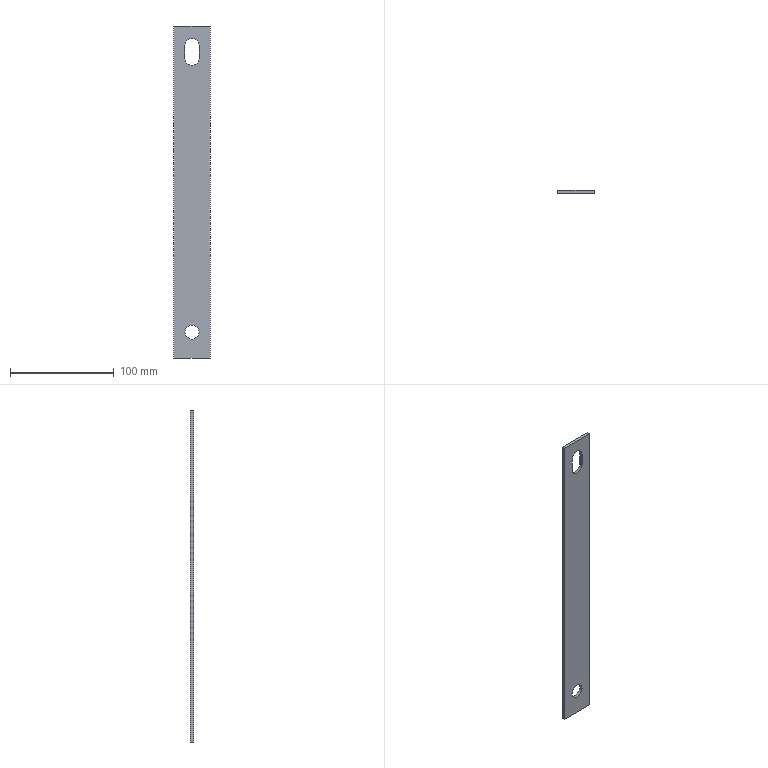Part | NX | features solid 2 | 1 solid | 11 faces | box 35 x 3 x 320 mm | volume 32235 mm3 | plane 8 | cylinder 3 | commonest cylinder face diameters 13.5 x3
STEP:
#1=CARTESIAN_POINT('',(957.5,320.,-165.));
#2=VERTEX_POINT('',#1);
#3=CARTESIAN_POINT('',(922.5,320.,-165.));
#4=VERTEX_POINT('',#3);
#5=CARTESIAN_POINT('',(957.5,320.,-165.));
#6=DIRECTION('',(-1.,0.,0.));
#7=VECTOR('',#6,1000.);
#8=LINE('',#5,#7);
#9=EDGE_CURVE('',#2,#4,#8,.T.);
#10=ORIENTED_EDGE('',*,*,#9,.T.);
#11=CARTESIAN_POINT('',(922.5,323.,-165.));
#12=VERTEX_POINT('',#11);
#13=CARTESIAN_POINT('',(922.5,323.,-165.));
#14=DIRECTION('',(0.,-1.,0.));
#15=VECTOR('',#14,1000.);
#16=LINE('',#13,#15);
#17=EDGE_CURVE('',#12,#4,#16,.T.);
#18=ORIENTED_EDGE('',*,*,#17,.F.);
#19=CARTESIAN_POINT('',(957.5,323.,-165.));
#20=VERTEX_POINT('',#19);
#21=CARTESIAN_POINT('',(957.5,323.,-165.));
#22=DIRECTION('',(-1.,0.,0.));
#23=VECTOR('',#22,1000.);
#24=LINE('',#21,#23);
#25=EDGE_CURVE('',#20,#12,#24,.T.);
#26=ORIENTED_EDGE('',*,*,#25,.F.);
#27=CARTESIAN_POINT('',(957.5,323.,-165.));
#28=DIRECTION('',(0.,-1.,0.));
#29=VECTOR('',#28,1000.);
#30=LINE('',#27,#29);
#31=EDGE_CURVE('',#20,#2,#30,.T.);
#32=ORIENTED_EDGE('',*,*,#31,.T.);
#33=EDGE_LOOP('',(#10,#18,#26,#32));
#34=FACE_BOUND('',#33,.T.);
#35=CARTESIAN_POINT('',(957.5,323.,-165.));
#36=DIRECTION('',(0.,0.,-1.));
#37=DIRECTION('',(0.,1.,0.));
#38=AXIS2_PLACEMENT_3D('',#35,#36,#37);
#39=PLANE('',#38);
#40=ADVANCED_FACE('',(#34),#39,.T.);
#41=CARTESIAN_POINT('',(933.25,323.,-140.));
#42=VERTEX_POINT('',#41);
#43=CARTESIAN_POINT('',(940.,323.,-140.));
#44=DIRECTION('',(0.,1.,0.));
#45=DIRECTION('',(-1.,0.,0.));
#46=AXIS2_PLACEMENT_3D('',#43,#44,#45);
#47=CIRCLE('',#46,6.75);
#48=EDGE_CURVE('',#42,#42,#47,.T.);
#49=ORIENTED_EDGE('',*,*,#48,.T.);
#50=EDGE_LOOP('',(#49));
#51=FACE_BOUND('',#50,.T.);
#52=CARTESIAN_POINT('',(933.25,320.,-140.));
#53=VERTEX_POINT('',#52);
#54=CARTESIAN_POINT('',(940.,320.,-140.));
#55=DIRECTION('',(0.,1.,0.));
#56=DIRECTION('',(-1.,0.,0.));
#57=AXIS2_PLACEMENT_3D('',#54,#55,#56);
#58=CIRCLE('',#57,6.75);
#59=EDGE_CURVE('',#53,#53,#58,.T.);
#60=ORIENTED_EDGE('',*,*,#59,.F.);
#61=EDGE_LOOP('',(#60));
#62=FACE_BOUND('',#61,.T.);
#63=CARTESIAN_POINT('',(940.,323.,-140.));
#64=DIRECTION('',(0.,-1.,0.));
#65=DIRECTION('',(-1.,0.,0.));
#66=AXIS2_PLACEMENT_3D('',#63,#64,#65);
#67=CYLINDRICAL_SURFACE('',#66,6.75);
#68=ADVANCED_FACE('',(#51,#62),#67,.F.);
#69=CARTESIAN_POINT('',(922.5,320.,155.));
#70=VERTEX_POINT('',#69);
#71=CARTESIAN_POINT('',(957.5,320.,155.));
#72=VERTEX_POINT('',#71);
#73=CARTESIAN_POINT('',(922.5,320.,155.));
#74=DIRECTION('',(1.,0.,0.));
#75=VECTOR('',#74,1000.);
#76=LINE('',#73,#75);
#77=EDGE_CURVE('',#70,#72,#76,.T.);
#78=ORIENTED_EDGE('',*,*,#77,.F.);
#79=CARTESIAN_POINT('',(922.5,320.,-85.));
#80=DIRECTION('',(0.,0.,1.));
#81=VECTOR('',#80,1000.);
#82=LINE('',#79,#81);
#83=EDGE_CURVE('',#4,#70,#82,.T.);
#84=ORIENTED_EDGE('',*,*,#83,.F.);
#85=ORIENTED_EDGE('',*,*,#9,.F.);
#86=CARTESIAN_POINT('',(957.5,320.,215.));
#87=DIRECTION('',(0.,0.,-1.));
#88=VECTOR('',#87,1000.);
#89=LINE('',#86,#88);
#90=EDGE_CURVE('',#72,#2,#89,.T.);
#91=ORIENTED_EDGE('',*,*,#90,.F.);
#92=EDGE_LOOP('',(#78,#84,#85,#91));
#93=FACE_BOUND('',#92,.T.);
#94=ORIENTED_EDGE('',*,*,#59,.T.);
#95=EDGE_LOOP('',(#94));
#96=FACE_BOUND('',#95,.T.);
#97=CARTESIAN_POINT('',(933.25,320.,136.25));
#98=VERTEX_POINT('',#97);
#99=CARTESIAN_POINT('',(946.75,320.,136.25));
#100=VERTEX_POINT('',#99);
#101=CARTESIAN_POINT('',(940.,320.,136.25));
#102=DIRECTION('',(0.,1.,0.));
#103=DIRECTION('',(-1.,0.,0.));
#104=AXIS2_PLACEMENT_3D('',#101,#102,#103);
#105=CIRCLE('',#104,6.75);
#106=EDGE_CURVE('',#98,#100,#105,.T.);
#107=ORIENTED_EDGE('',*,*,#106,.T.);
#108=CARTESIAN_POINT('',(946.75,320.,123.75));
#109=VERTEX_POINT('',#108);
#110=CARTESIAN_POINT('',(946.75,320.,123.75));
#111=DIRECTION('',(0.,0.,1.));
#112=VECTOR('',#111,1000.);
#113=LINE('',#110,#112);
#114=EDGE_CURVE('',#109,#100,#113,.T.);
#115=ORIENTED_EDGE('',*,*,#114,.F.);
#116=CARTESIAN_POINT('',(933.25,320.,123.75));
#117=VERTEX_POINT('',#116);
#118=CARTESIAN_POINT('',(940.,320.,123.75));
#119=DIRECTION('',(0.,1.,0.));
#120=DIRECTION('',(-1.,0.,0.));
#121=AXIS2_PLACEMENT_3D('',#118,#119,#120);
#122=CIRCLE('',#121,6.75);
#123=EDGE_CURVE('',#109,#117,#122,.T.);
#124=ORIENTED_EDGE('',*,*,#123,.T.);
#125=CARTESIAN_POINT('',(933.25,320.,136.25));
#126=DIRECTION('',(0.,0.,-1.));
#127=VECTOR('',#126,1000.);
#128=LINE('',#125,#127);
#129=EDGE_CURVE('',#98,#117,#128,.T.);
#130=ORIENTED_EDGE('',*,*,#129,.F.);
#131=EDGE_LOOP('',(#107,#115,#124,#130));
#132=FACE_BOUND('',#131,.T.);
#133=CARTESIAN_POINT('',(922.5,320.,215.));
#134=DIRECTION('',(0.,-1.,0.));
#135=DIRECTION('',(-1.,0.,0.));
#136=AXIS2_PLACEMENT_3D('',#133,#134,#135);
#137=PLANE('',#136);
#138=ADVANCED_FACE('',(#93,#96,#132),#137,.T.);
#139=CARTESIAN_POINT('',(957.5,323.,155.));
#140=VERTEX_POINT('',#139);
#141=CARTESIAN_POINT('',(957.5,323.,215.));
#142=DIRECTION('',(0.,0.,-1.));
#143=VECTOR('',#142,1000.);
#144=LINE('',#141,#143);
#145=EDGE_CURVE('',#140,#20,#144,.T.);
#146=ORIENTED_EDGE('',*,*,#145,.T.);
#147=ORIENTED_EDGE('',*,*,#25,.T.);
#148=CARTESIAN_POINT('',(922.5,323.,155.));
#149=VERTEX_POINT('',#148);
#150=CARTESIAN_POINT('',(922.5,323.,-85.));
#151=DIRECTION('',(0.,0.,1.));
#152=VECTOR('',#151,1000.);
#153=LINE('',#150,#152);
#154=EDGE_CURVE('',#12,#149,#153,.T.);
#155=ORIENTED_EDGE('',*,*,#154,.T.);
#156=CARTESIAN_POINT('',(922.5,323.,155.));
#157=DIRECTION('',(1.,0.,0.));
#158=VECTOR('',#157,1000.);
#159=LINE('',#156,#158);
#160=EDGE_CURVE('',#149,#140,#159,.T.);
#161=ORIENTED_EDGE('',*,*,#160,.T.);
#162=EDGE_LOOP('',(#146,#147,#155,#161));
#163=FACE_BOUND('',#162,.T.);
#164=ORIENTED_EDGE('',*,*,#48,.F.);
#165=EDGE_LOOP('',(#164));
#166=FACE_BOUND('',#165,.T.);
#167=CARTESIAN_POINT('',(933.25,323.,136.25));
#168=VERTEX_POINT('',#167);
#169=CARTESIAN_POINT('',(946.75,323.,136.25));
#170=VERTEX_POINT('',#169);
#171=CARTESIAN_POINT('',(940.,323.,136.25));
#172=DIRECTION('',(0.,1.,0.));
#173=DIRECTION('',(-1.,0.,0.));
#174=AXIS2_PLACEMENT_3D('',#171,#172,#173);
#175=CIRCLE('',#174,6.75);
#176=EDGE_CURVE('',#168,#170,#175,.T.);
#177=ORIENTED_EDGE('',*,*,#176,.F.);
#178=CARTESIAN_POINT('',(933.25,323.,123.75));
#179=VERTEX_POINT('',#178);
#180=CARTESIAN_POINT('',(933.25,323.,136.25));
#181=DIRECTION('',(0.,0.,-1.));
#182=VECTOR('',#181,1000.);
#183=LINE('',#180,#182);
#184=EDGE_CURVE('',#168,#179,#183,.T.);
#185=ORIENTED_EDGE('',*,*,#184,.T.);
#186=CARTESIAN_POINT('',(946.75,323.,123.75));
#187=VERTEX_POINT('',#186);
#188=CARTESIAN_POINT('',(940.,323.,123.75));
#189=DIRECTION('',(0.,1.,0.));
#190=DIRECTION('',(-1.,0.,0.));
#191=AXIS2_PLACEMENT_3D('',#188,#189,#190);
#192=CIRCLE('',#191,6.75);
#193=EDGE_CURVE('',#187,#179,#192,.T.);
#194=ORIENTED_EDGE('',*,*,#193,.F.);
#195=CARTESIAN_POINT('',(946.75,323.,123.75));
#196=DIRECTION('',(0.,0.,1.));
#197=VECTOR('',#196,1000.);
#198=LINE('',#195,#197);
#199=EDGE_CURVE('',#187,#170,#198,.T.);
#200=ORIENTED_EDGE('',*,*,#199,.T.);
#201=EDGE_LOOP('',(#177,#185,#194,#200));
#202=FACE_BOUND('',#201,.T.);
#203=CARTESIAN_POINT('',(922.5,323.,215.));
#204=DIRECTION('',(0.,-1.,0.));
#205=DIRECTION('',(-1.,0.,0.));
#206=AXIS2_PLACEMENT_3D('',#203,#204,#205);
#207=PLANE('',#206);
#208=ADVANCED_FACE('',(#163,#166,#202),#207,.F.);
#209=ORIENTED_EDGE('',*,*,#90,.T.);
#210=ORIENTED_EDGE('',*,*,#31,.F.);
#211=ORIENTED_EDGE('',*,*,#145,.F.);
#212=CARTESIAN_POINT('',(957.5,323.,155.));
#213=DIRECTION('',(0.,-1.,0.));
#214=VECTOR('',#213,1000.);
#215=LINE('',#212,#214);
#216=EDGE_CURVE('',#140,#72,#215,.T.);
#217=ORIENTED_EDGE('',*,*,#216,.T.);
#218=EDGE_LOOP('',(#209,#210,#211,#217));
#219=FACE_BOUND('',#218,.T.);
#220=CARTESIAN_POINT('',(957.5,323.,215.));
#221=DIRECTION('',(1.,0.,0.));
#222=DIRECTION('',(0.,0.,-1.));
#223=AXIS2_PLACEMENT_3D('',#220,#221,#222);
#224=PLANE('',#223);
#225=ADVANCED_FACE('',(#219),#224,.T.);
#226=CARTESIAN_POINT('',(922.5,323.,155.));
#227=DIRECTION('',(0.,-1.,0.));
#228=VECTOR('',#227,1000.);
#229=LINE('',#226,#228);
#230=EDGE_CURVE('',#149,#70,#229,.T.);
#231=ORIENTED_EDGE('',*,*,#230,.F.);
#232=ORIENTED_EDGE('',*,*,#154,.F.);
#233=ORIENTED_EDGE('',*,*,#17,.T.);
#234=ORIENTED_EDGE('',*,*,#83,.T.);
#235=EDGE_LOOP('',(#231,#232,#233,#234));
#236=FACE_BOUND('',#235,.T.);
#237=CARTESIAN_POINT('',(922.5,323.,-85.));
#238=DIRECTION('',(-1.,0.,0.));
#239=DIRECTION('',(0.,0.,1.));
#240=AXIS2_PLACEMENT_3D('',#237,#238,#239);
#241=PLANE('',#240);
#242=ADVANCED_FACE('',(#236),#241,.T.);
#243=ORIENTED_EDGE('',*,*,#106,.F.);
#244=CARTESIAN_POINT('',(933.25,323.,136.25));
#245=DIRECTION('',(0.,-1.,0.));
#246=VECTOR('',#245,1000.);
#247=LINE('',#244,#246);
#248=EDGE_CURVE('',#168,#98,#247,.T.);
#249=ORIENTED_EDGE('',*,*,#248,.F.);
#250=ORIENTED_EDGE('',*,*,#176,.T.);
#251=CARTESIAN_POINT('',(946.75,323.,136.25));
#252=DIRECTION('',(0.,-1.,0.));
#253=VECTOR('',#252,1000.);
#254=LINE('',#251,#253);
#255=EDGE_CURVE('',#170,#100,#254,.T.);
#256=ORIENTED_EDGE('',*,*,#255,.T.);
#257=EDGE_LOOP('',(#243,#249,#250,#256));
#258=FACE_BOUND('',#257,.T.);
#259=CARTESIAN_POINT('',(940.,323.,136.25));
#260=DIRECTION('',(0.,-1.,0.));
#261=DIRECTION('',(-1.,0.,0.));
#262=AXIS2_PLACEMENT_3D('',#259,#260,#261);
#263=CYLINDRICAL_SURFACE('',#262,6.75);
#264=ADVANCED_FACE('',(#258),#263,.F.);
#265=ORIENTED_EDGE('',*,*,#129,.T.);
#266=CARTESIAN_POINT('',(933.25,323.,123.75));
#267=DIRECTION('',(0.,-1.,0.));
#268=VECTOR('',#267,1000.);
#269=LINE('',#266,#268);
#270=EDGE_CURVE('',#179,#117,#269,.T.);
#271=ORIENTED_EDGE('',*,*,#270,.F.);
#272=ORIENTED_EDGE('',*,*,#184,.F.);
#273=ORIENTED_EDGE('',*,*,#248,.T.);
#274=EDGE_LOOP('',(#265,#271,#272,#273));
#275=FACE_BOUND('',#274,.T.);
#276=CARTESIAN_POINT('',(933.25,323.,136.25));
#277=DIRECTION('',(1.,0.,0.));
#278=DIRECTION('',(0.,-1.,0.));
#279=AXIS2_PLACEMENT_3D('',#276,#277,#278);
#280=PLANE('',#279);
#281=ADVANCED_FACE('',(#275),#280,.T.);
#282=ORIENTED_EDGE('',*,*,#123,.F.);
#283=CARTESIAN_POINT('',(946.75,323.,123.75));
#284=DIRECTION('',(0.,-1.,0.));
#285=VECTOR('',#284,1000.);
#286=LINE('',#283,#285);
#287=EDGE_CURVE('',#187,#109,#286,.T.);
#288=ORIENTED_EDGE('',*,*,#287,.F.);
#289=ORIENTED_EDGE('',*,*,#193,.T.);
#290=ORIENTED_EDGE('',*,*,#270,.T.);
#291=EDGE_LOOP('',(#282,#288,#289,#290));
#292=FACE_BOUND('',#291,.T.);
#293=CARTESIAN_POINT('',(940.,323.,123.75));
#294=DIRECTION('',(0.,-1.,0.));
#295=DIRECTION('',(-1.,0.,0.));
#296=AXIS2_PLACEMENT_3D('',#293,#294,#295);
#297=CYLINDRICAL_SURFACE('',#296,6.75);
#298=ADVANCED_FACE('',(#292),#297,.F.);
#299=ORIENTED_EDGE('',*,*,#77,.T.);
#300=ORIENTED_EDGE('',*,*,#216,.F.);
#301=ORIENTED_EDGE('',*,*,#160,.F.);
#302=ORIENTED_EDGE('',*,*,#230,.T.);
#303=EDGE_LOOP('',(#299,#300,#301,#302));
#304=FACE_BOUND('',#303,.T.);
#305=CARTESIAN_POINT('',(922.5,323.,155.));
#306=DIRECTION('',(0.,0.,1.));
#307=DIRECTION('',(0.,-1.,0.));
#308=AXIS2_PLACEMENT_3D('',#305,#306,#307);
#309=PLANE('',#308);
#310=ADVANCED_FACE('',(#304),#309,.T.);
#311=ORIENTED_EDGE('',*,*,#114,.T.);
#312=ORIENTED_EDGE('',*,*,#255,.F.);
#313=ORIENTED_EDGE('',*,*,#199,.F.);
#314=ORIENTED_EDGE('',*,*,#287,.T.);
#315=EDGE_LOOP('',(#311,#312,#313,#314));
#316=FACE_BOUND('',#315,.T.);
#317=CARTESIAN_POINT('',(946.75,323.,123.75));
#318=DIRECTION('',(-1.,0.,0.));
#319=DIRECTION('',(0.,1.,0.));
#320=AXIS2_PLACEMENT_3D('',#317,#318,#319);
#321=PLANE('',#320);
#322=ADVANCED_FACE('',(#316),#321,.T.);
#323=CLOSED_SHELL('',(#40,#68,#138,#208,#225,#242,#264,#281,#298,#310,#322));
#324=MANIFOLD_SOLID_BREP('',#323);
#325=(LENGTH_UNIT()NAMED_UNIT(*)SI_UNIT(.MILLI.,.METRE.));
#326=UNCERTAINTY_MEASURE_WITH_UNIT(LENGTH_MEASURE(0.00001),#325,'','');
#327=(NAMED_UNIT(*)PLANE_ANGLE_UNIT()SI_UNIT($,.RADIAN.));
#328=(NAMED_UNIT(*)SI_UNIT($,.STERADIAN.)SOLID_ANGLE_UNIT());
#329=(GEOMETRIC_REPRESENTATION_CONTEXT(3)GLOBAL_UNCERTAINTY_ASSIGNED_CONTEXT((#326))GLOBAL_UNIT_ASSIGNED_CONTEXT((#325,#327,#328))REPRESENTATION_CONTEXT('',''));
#330=ADVANCED_BREP_SHAPE_REPRESENTATION('',(#324),#329);